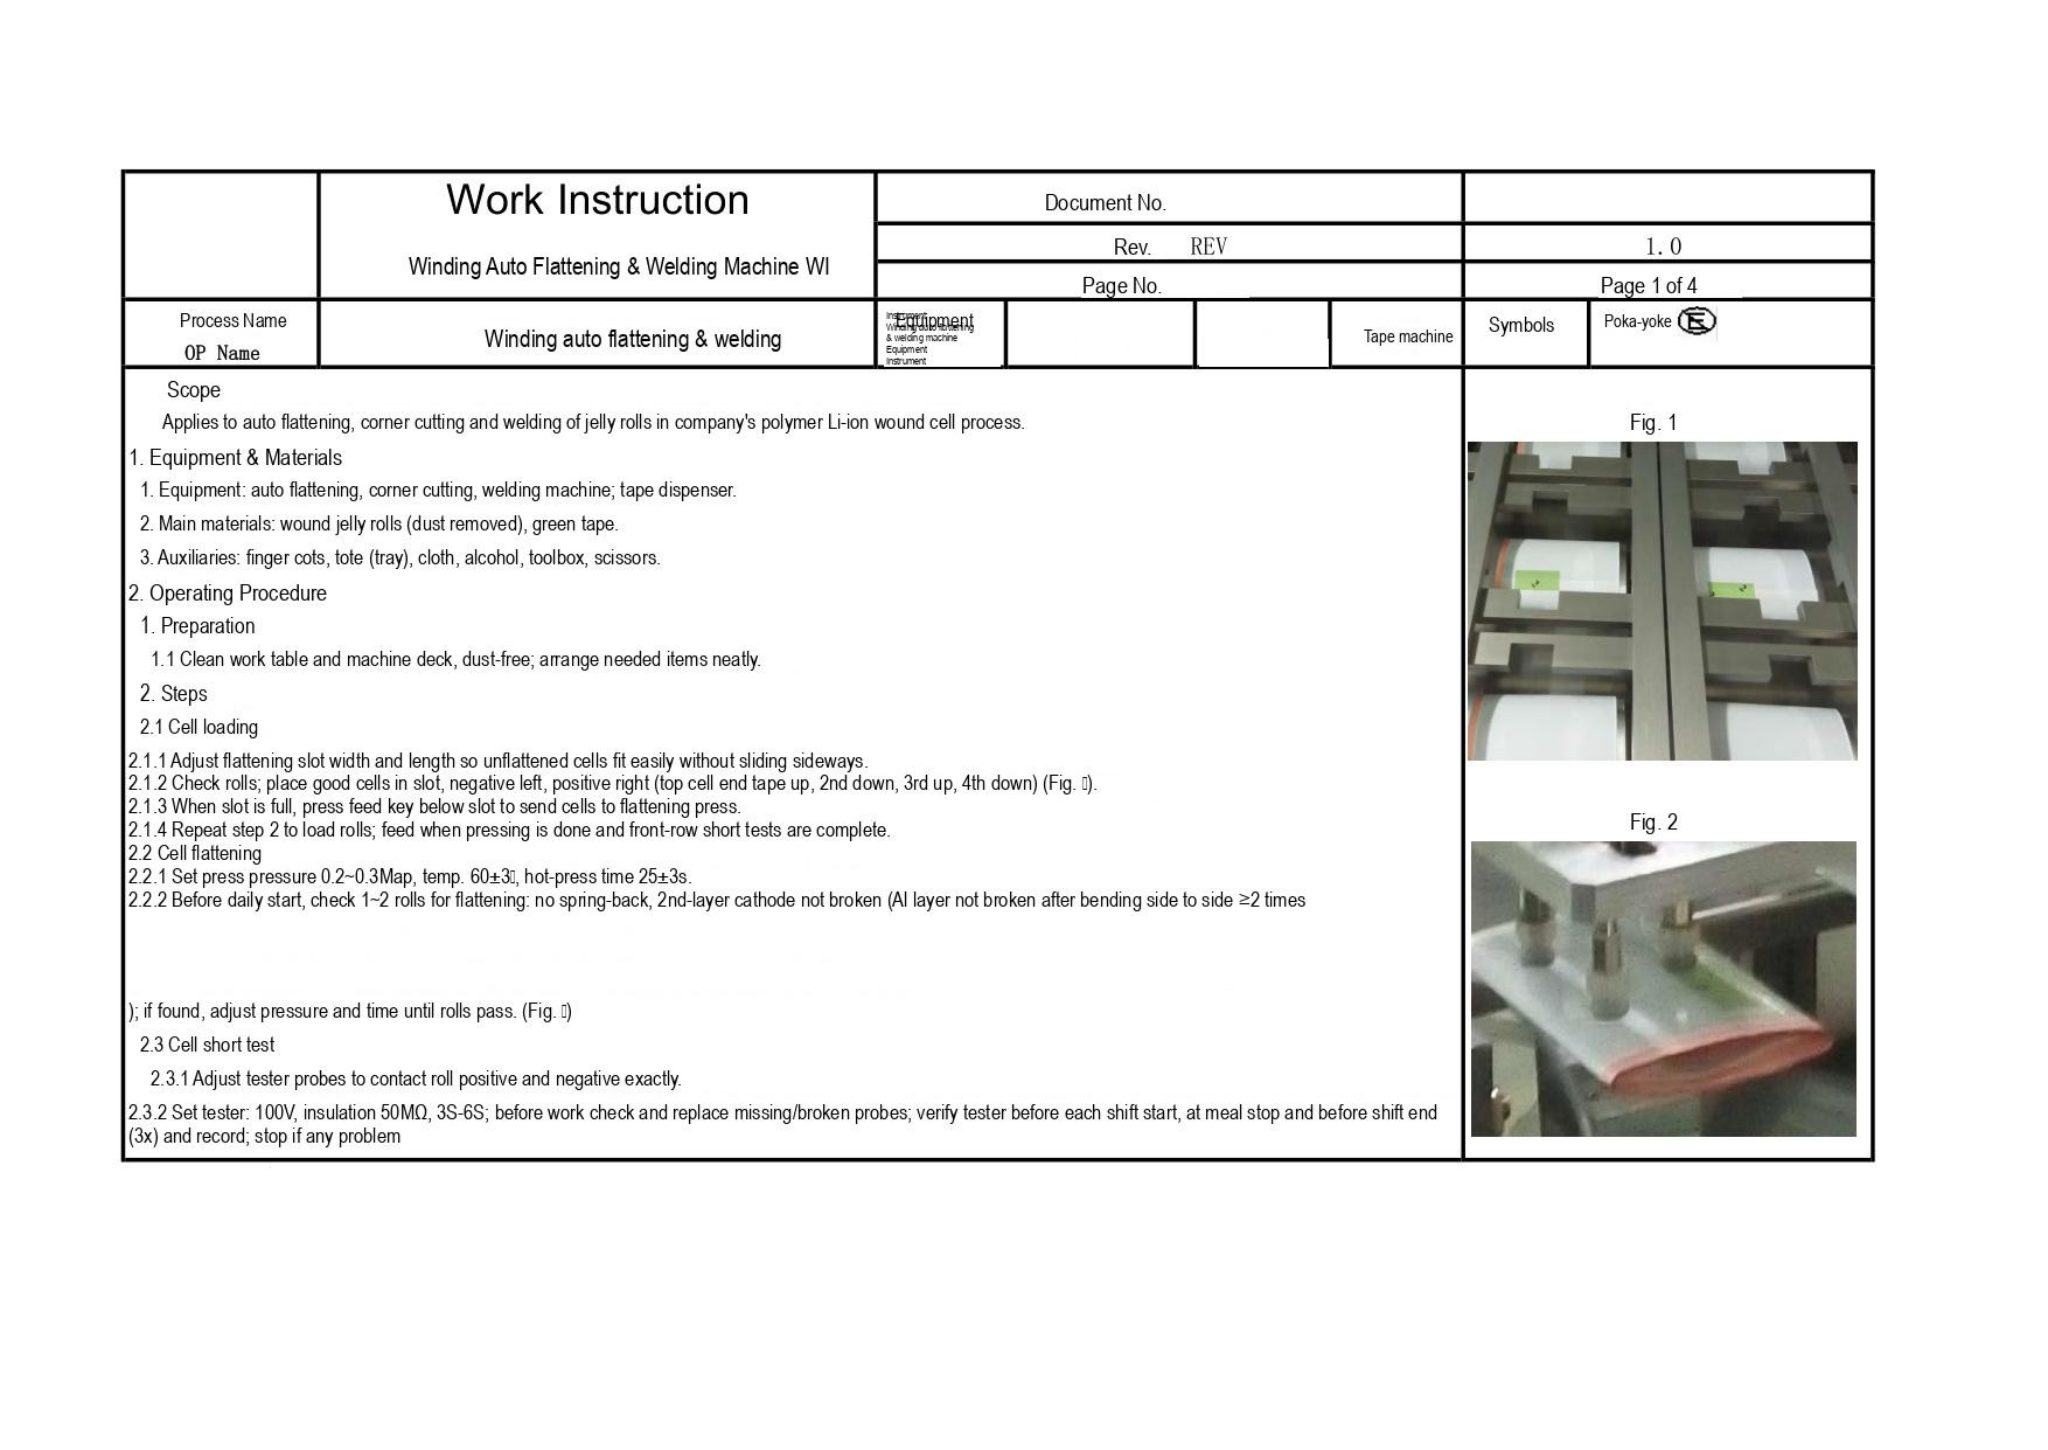| | Work Instruction<br>Winding Auto Flattening & Welding Machine WI | Document No. | |
|---|---|---|---|
| | | Rev. REV | 1.0 |
| | | Page No. | Page 1 of 4 |

| Process Name<br>OP Name | Winding auto flattening & welding | Equipment<br>Instrument<br>Winding auto flattening & welding machine<br>Equipment<br>Instrument | | | Tape machine | Symbols | Poka-yoke |
|---|---|---|---|---|---|---|---|

Scope

Applies to auto flattening, corner cutting and welding of jelly rolls in company's polymer Li-ion wound cell process.

1. Equipment & Materials

1. Equipment: auto flattening, corner cutting, welding machine; tape dispenser.

2. Main materials: wound jelly rolls (dust removed), green tape.

3. Auxiliaries: finger cots, tote (tray), cloth, alcohol, toolbox, scissors.

2. Operating Procedure

1. Preparation

1.1 Clean work table and machine deck, dust-free; arrange needed items neatly.

2. Steps

2.1 Cell loading

2.1.1 Adjust flattening slot width and length so unflattened cells fit easily without sliding sideways.
2.1.2 Check rolls; place good cells in slot, negative left, positive right (top cell end tape up, 2nd down, 3rd up, 4th down) (Fig. ).
2.1.3 When slot is full, press feed key below slot to send cells to flattening press.
2.1.4 Repeat step 2 to load rolls; feed when pressing is done and front-row short tests are complete.
2.2 Cell flattening
2.2.1 Set press pressure 0.2~0.3Map, temp. 60±3, hot-press time 25±3s.
2.2.2 Before daily start, check 1~2 rolls for flattening: no spring-back, 2nd-layer cathode not broken (Al layer not broken after bending side to side ≥2 times

); if found, adjust pressure and time until rolls pass. (Fig. )

2.3 Cell short test

2.3.1 Adjust tester probes to contact roll positive and negative exactly.

2.3.2 Set tester: 100V, insulation 50MΩ, 3S-6S; before work check and replace missing/broken probes; verify tester before each shift start, at meal stop and before shift end (3x) and record; stop if any problem

Fig. 1

Fig. 2
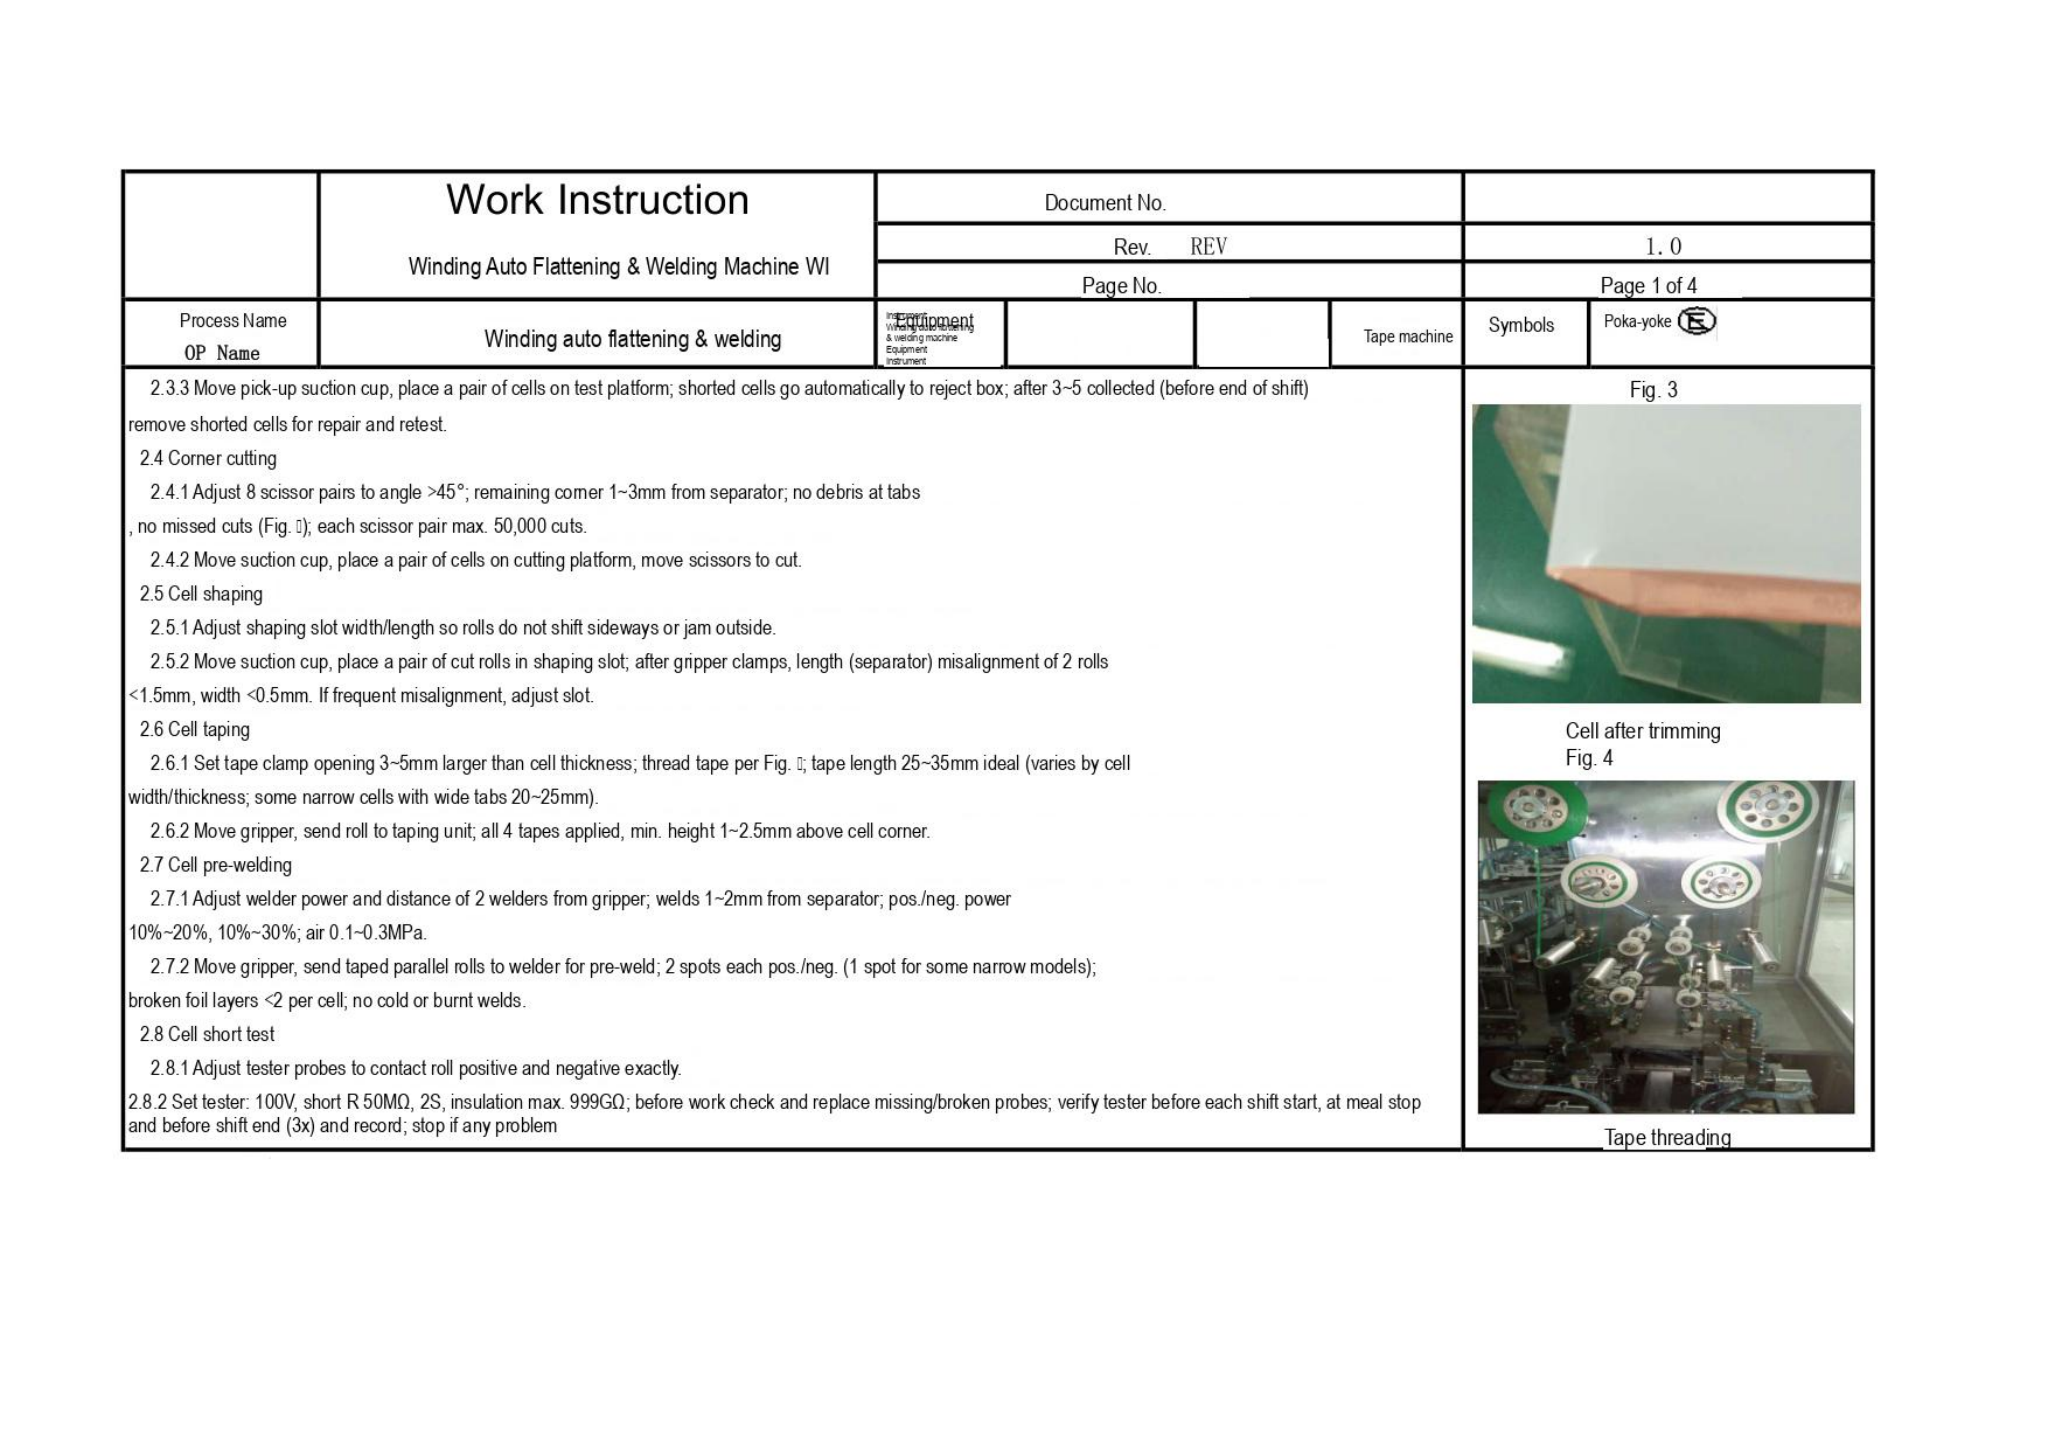| | Work Instruction<br>Winding Auto Flattening & Welding Machine WI | Document No. | | | | | |
|---|---|---|---|---|---|---|---|
| | | Rev. REV | | | | 1.0 | |
| | | Page No. | | | | Page 1 of 4 | |
| Process Name<br>OP Name | Winding auto flattening & welding | Equipment | | | Tape machine | Symbols | Poka-yoke |

2.3.3 Move pick-up suction cup, place a pair of cells on test platform; shorted cells go automatically to reject box; after 3~5 collected (before end of shift) remove shorted cells for repair and retest.

2.4 Corner cutting

2.4.1 Adjust 8 scissor pairs to angle >45°; remaining corner 1~3mm from separator; no debris at tabs, no missed cuts (Fig. ); each scissor pair max. 50,000 cuts.

2.4.2 Move suction cup, place a pair of cells on cutting platform, move scissors to cut.

2.5 Cell shaping

2.5.1 Adjust shaping slot width/length so rolls do not shift sideways or jam outside.

2.5.2 Move suction cup, place a pair of cut rolls in shaping slot; after gripper clamps, length (separator) misalignment of 2 rolls <1.5mm, width <0.5mm. If frequent misalignment, adjust slot.

2.6 Cell taping

2.6.1 Set tape clamp opening 3~5mm larger than cell thickness; thread tape per Fig. ; tape length 25~35mm ideal (varies by cell width/thickness; some narrow cells with wide tabs 20~25mm).

2.6.2 Move gripper, send roll to taping unit; all 4 tapes applied, min. height 1~2.5mm above cell corner.

2.7 Cell pre-welding

2.7.1 Adjust welder power and distance of 2 welders from gripper; welds 1~2mm from separator; pos./neg. power 10%~20%, 10%~30%; air 0.1~0.3MPa.

2.7.2 Move gripper, send taped parallel rolls to welder for pre-weld; 2 spots each pos./neg. (1 spot for some narrow models); broken foil layers <2 per cell; no cold or burnt welds.

2.8 Cell short test

2.8.1 Adjust tester probes to contact roll positive and negative exactly.

2.8.2 Set tester: 100V, short R 50MΩ, 2S, insulation max. 999GΩ; before work check and replace missing/broken probes; verify tester before each shift start, at meal stop and before shift end (3x) and record; stop if any problem

Fig. 3

Cell after trimming

Fig. 4

Tape threading
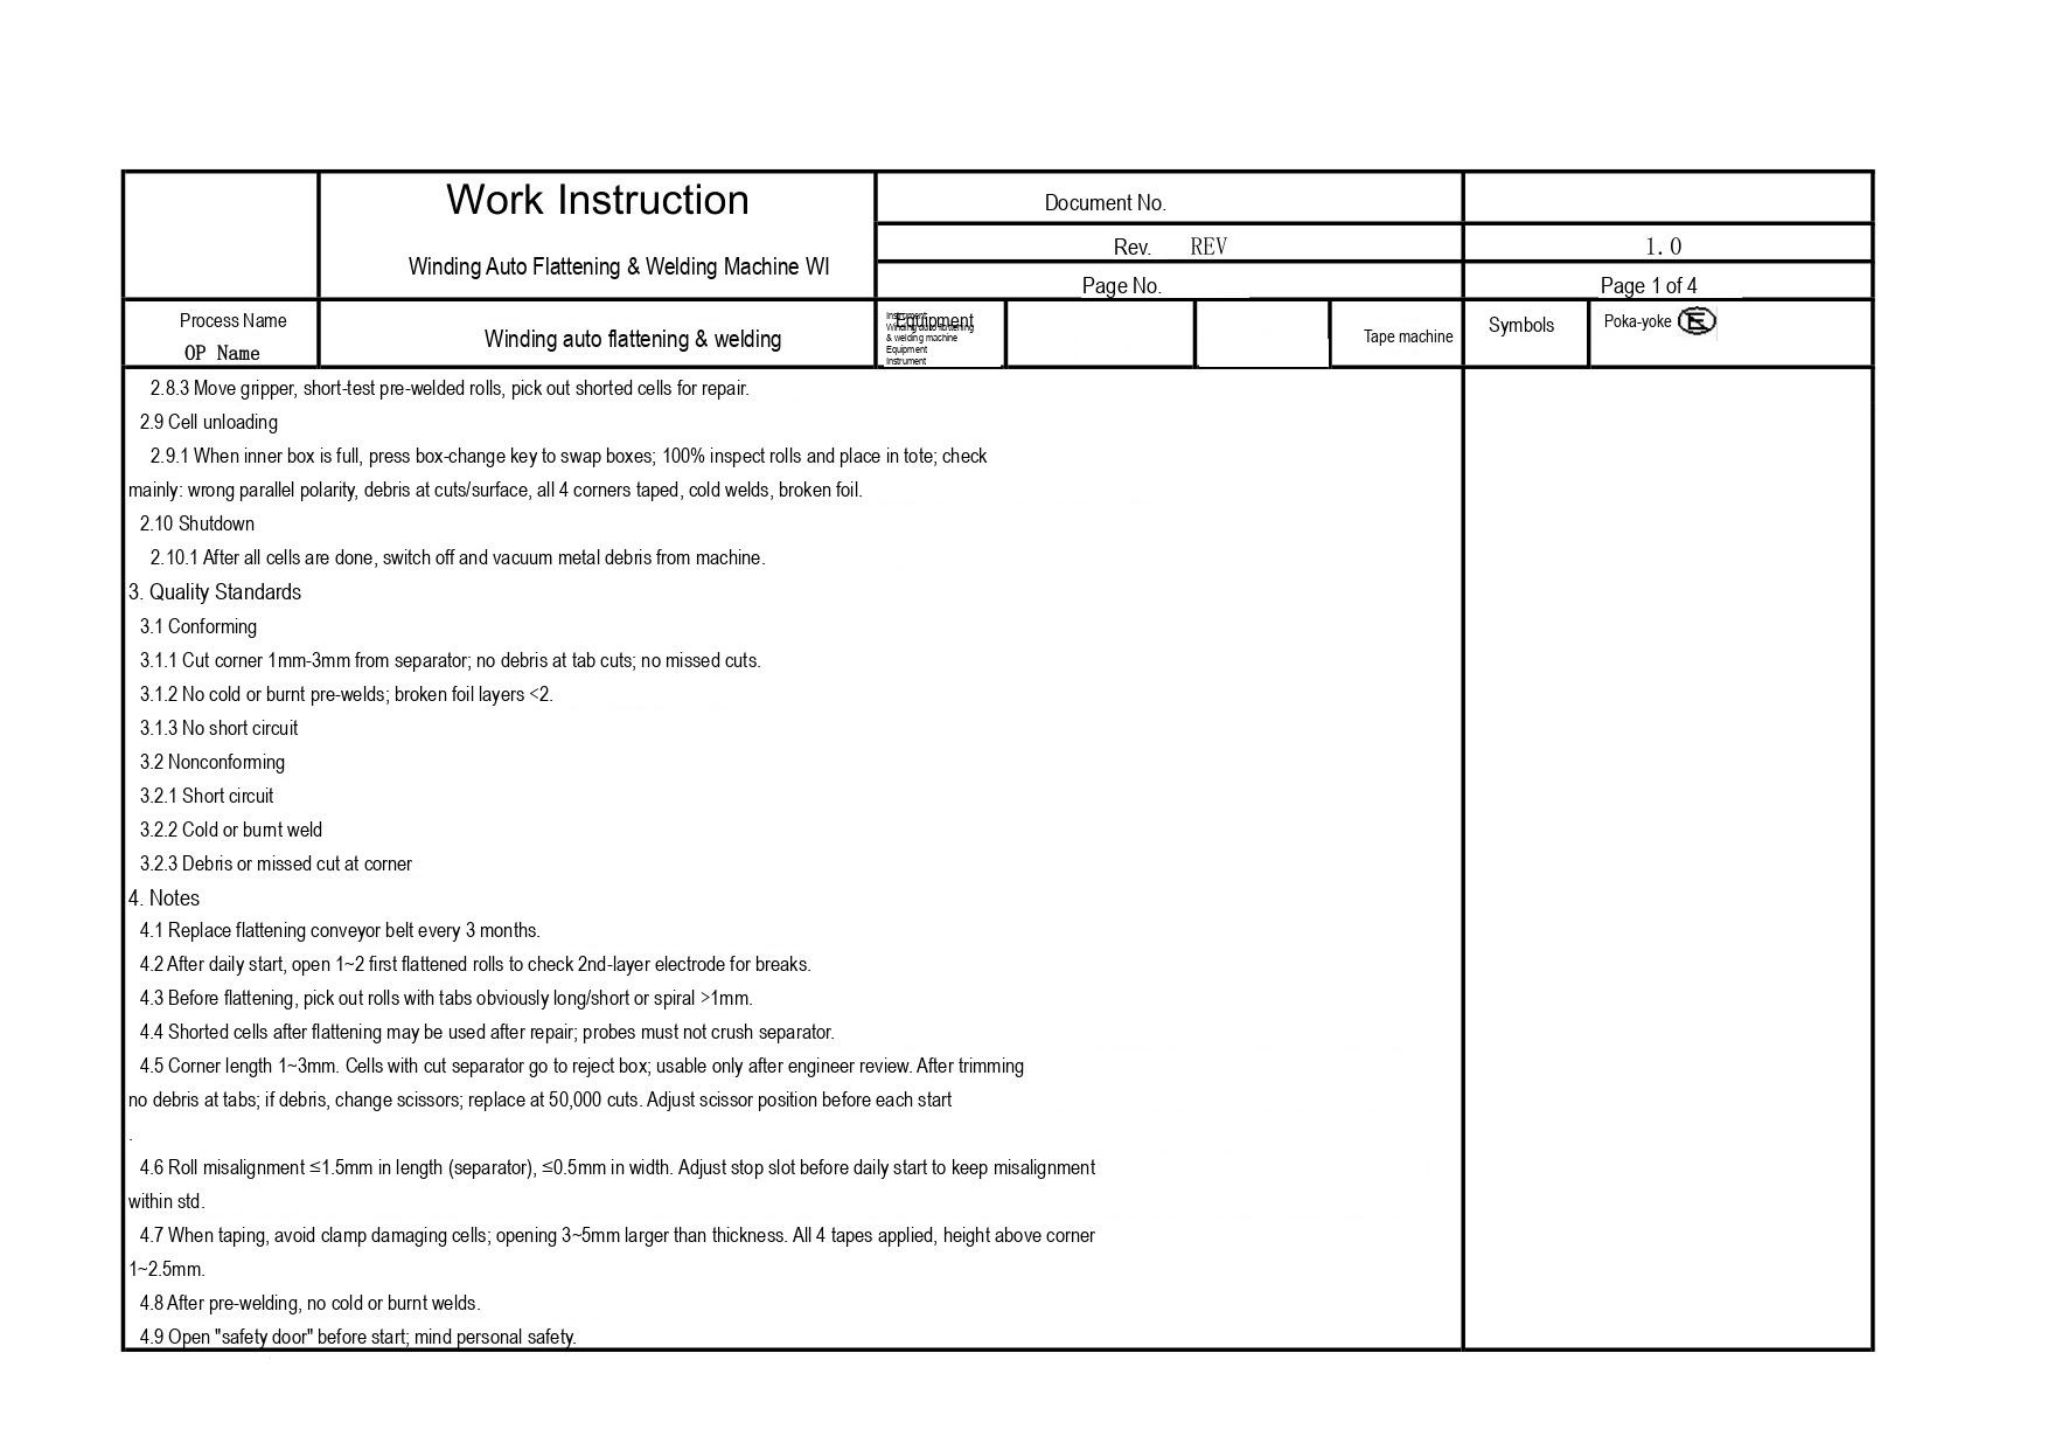| | Work Instruction<br>Winding Auto Flattening & Welding Machine WI | Document No. | | | | | |
|---|---|---|---|---|---|---|---|
| | | Rev. REV | | | | 1.0 | |
| | | Page No. | | | | Page 1 of 4 | |
| Process Name<br>OP Name | Winding auto flattening & welding | Equipment<br>Instrument<br>Winding auto flattening & welding machine<br>Equipment<br>Instrument | | | Tape machine | Symbols | Poka-yoke |

2.8.3 Move gripper, short-test pre-welded rolls, pick out shorted cells for repair.
2.9 Cell unloading
2.9.1 When inner box is full, press box-change key to swap boxes; 100% inspect rolls and place in tote; check mainly: wrong parallel polarity, debris at cuts/surface, all 4 corners taped, cold welds, broken foil.
2.10 Shutdown
2.10.1 After all cells are done, switch off and vacuum metal debris from machine.
3. Quality Standards
3.1 Conforming
3.1.1 Cut corner 1mm-3mm from separator; no debris at tab cuts; no missed cuts.
3.1.2 No cold or burnt pre-welds; broken foil layers <2.
3.1.3 No short circuit
3.2 Nonconforming
3.2.1 Short circuit
3.2.2 Cold or burnt weld
3.2.3 Debris or missed cut at corner
4. Notes
4.1 Replace flattening conveyor belt every 3 months.
4.2 After daily start, open 1~2 first flattened rolls to check 2nd-layer electrode for breaks.
4.3 Before flattening, pick out rolls with tabs obviously long/short or spiral >1mm.
4.4 Shorted cells after flattening may be used after repair; probes must not crush separator.
4.5 Corner length 1~3mm. Cells with cut separator go to reject box; usable only after engineer review. After trimming no debris at tabs; if debris, change scissors; replace at 50,000 cuts. Adjust scissor position before each start
.
4.6 Roll misalignment ≤1.5mm in length (separator), ≤0.5mm in width. Adjust stop slot before daily start to keep misalignment within std.
4.7 When taping, avoid clamp damaging cells; opening 3~5mm larger than thickness. All 4 tapes applied, height above corner 1~2.5mm.
4.8 After pre-welding, no cold or burnt welds.
4.9 Open "safety door" before start; mind personal safety.
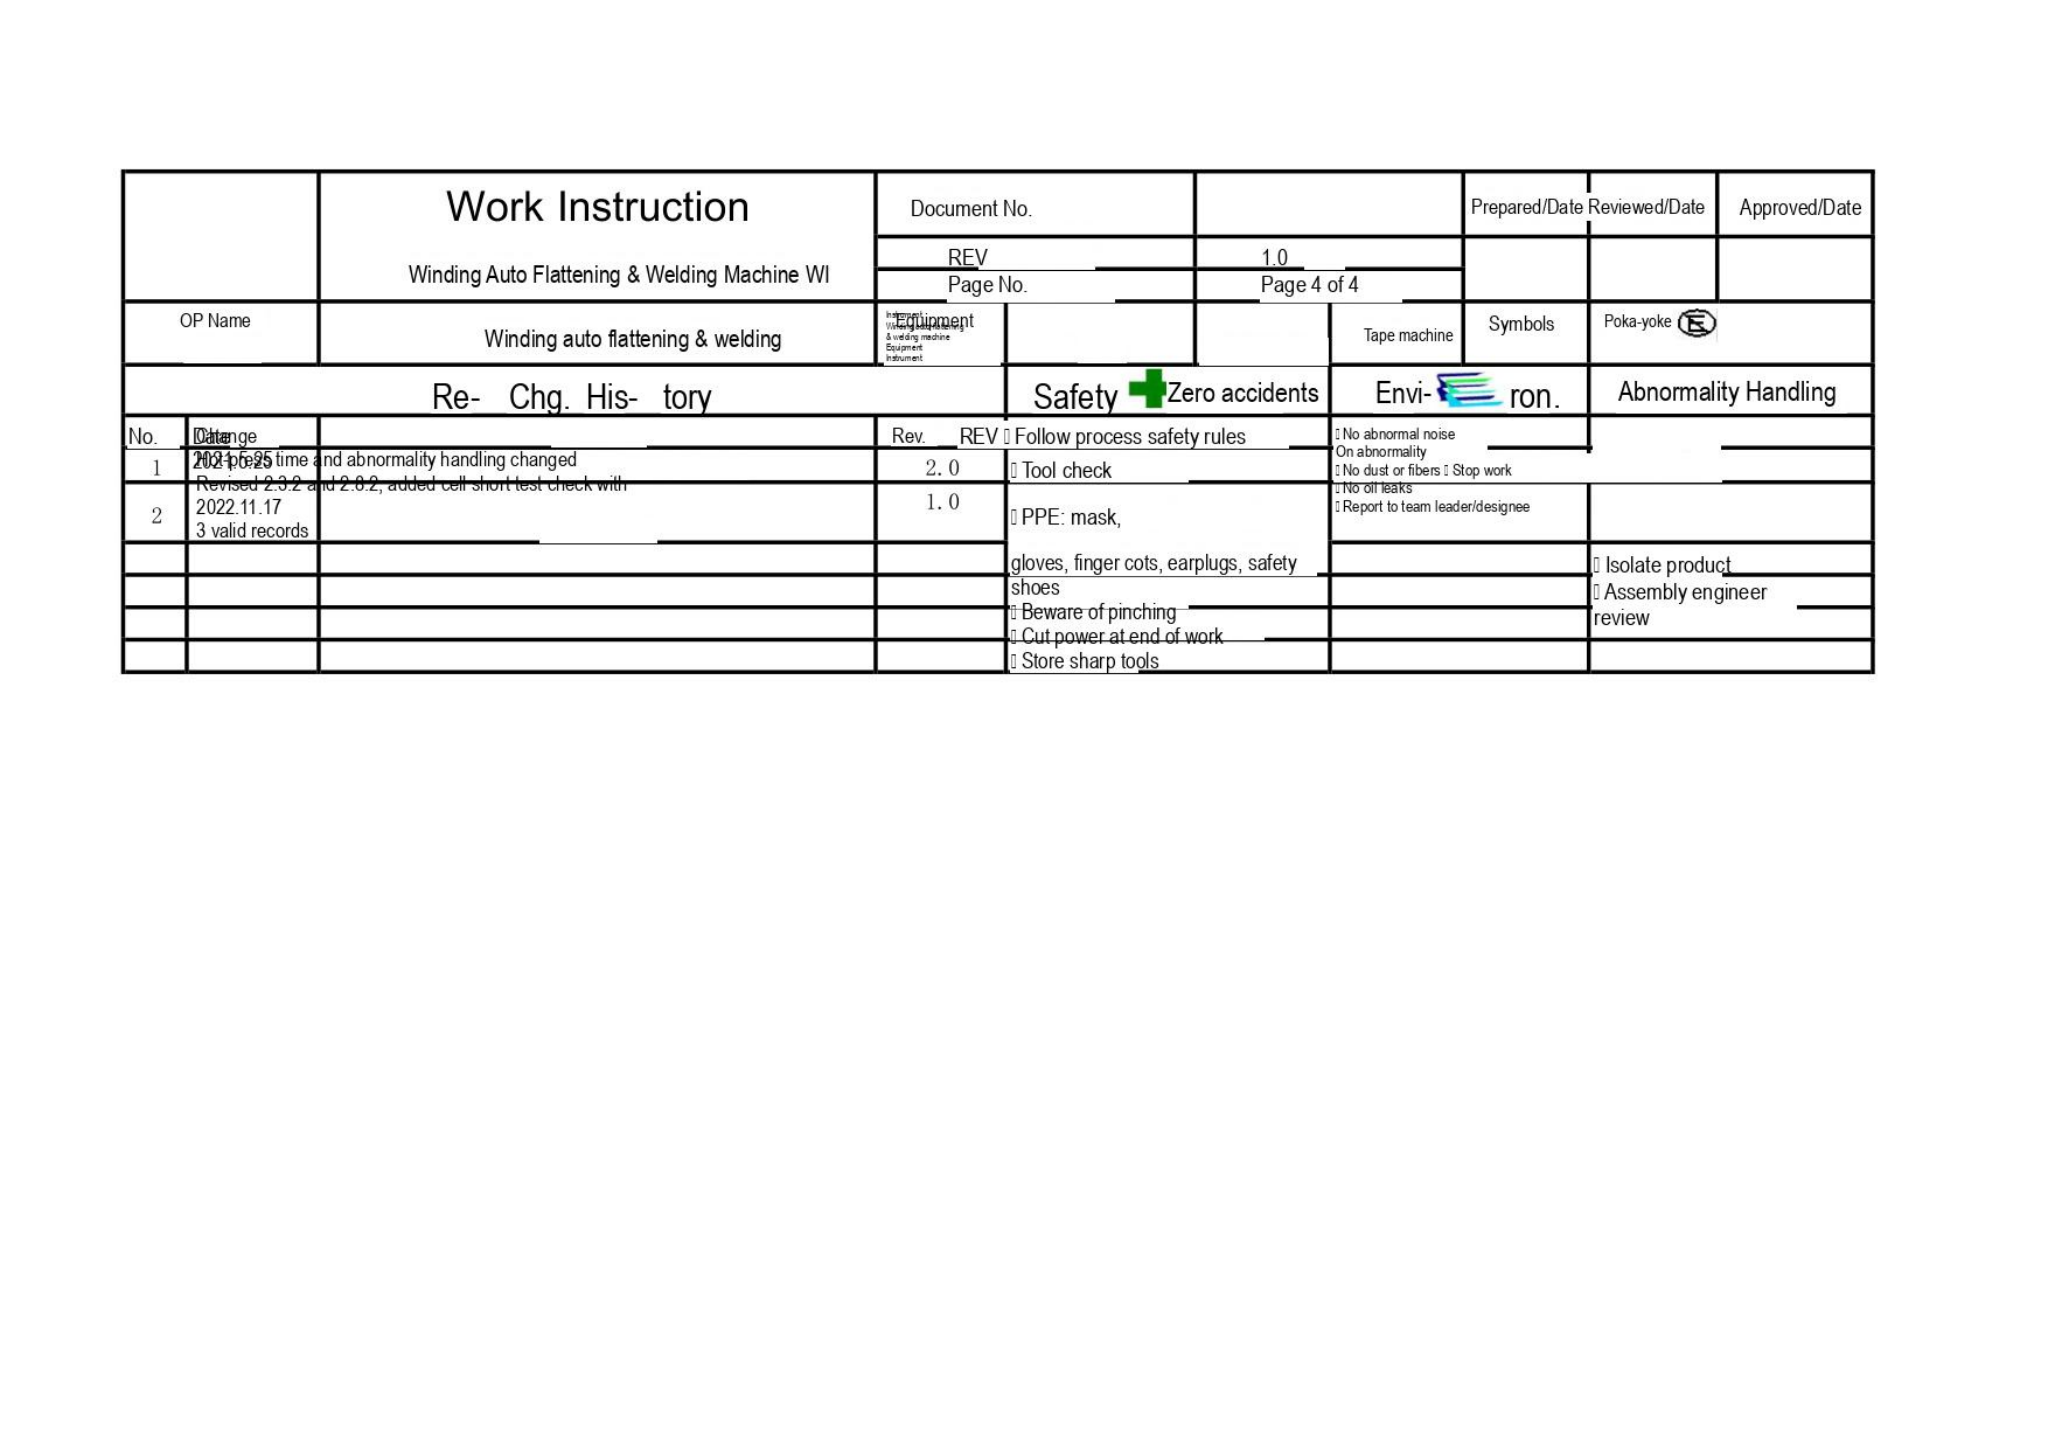| | Work Instruction<br>Winding Auto Flattening & Welding Machine WI | Document No. | | Prepared/Date | Reviewed/Date | Approved/Date |
|---|---|---|---|---|---|---|
| | | REV | 1.0 | | | |
| | | Page No. | Page 4 of 4 | | | |

| OP Name | Winding auto flattening & welding | Equipment<br>Instrument<br>Winding auto flattening & welding machine<br>Equipment<br>Instrument | | | Tape machine | Symbols | Poka-yoke |
|---|---|---|---|---|---|---|---|

| Re- Chg. His- tory | | | | Safety Zero accidents | Envi- ron. | Abnormality Handling |
|---|---|---|---|---|---|---|
| No. | Date | Change | Rev. REV | Follow process safety rules | No abnormal noise<br>On abnormality<br>No dust or fibers Stop work<br>No oil leaks<br>Report to team leader/designee | |
| 1 | 2021.5.25 | Process time and abnormality handling changed | 2.0 | Tool check | | |
| 2 | 2022.11.17 | Revised 2.3.2 and 2.8.2, added cell short test check with<br>3 valid records | 1.0 | PPE: mask, | | |
| | | | | gloves, finger cots, earplugs, safety shoes | | Isolate product<br>Assembly engineer review |
| | | | | Beware of pinching | | |
| | | | | Cut power at end of work | | |
| | | | | Store sharp tools | | |